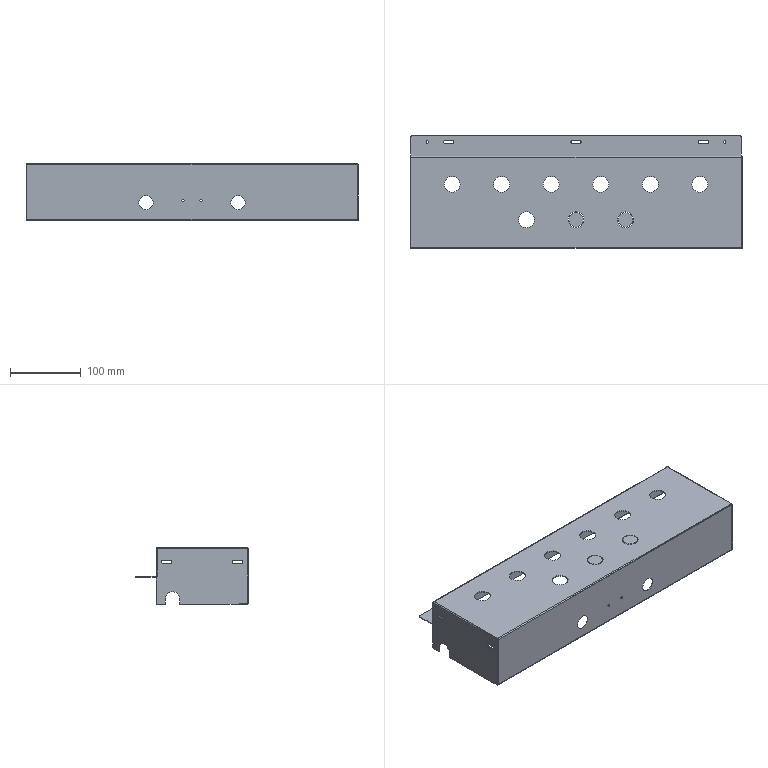Part | STEP file | 1 solid | 163 faces | box 469 x 158.8 x 80 mm | volume 180608 mm3 | cylinder 85 | plane 78 | commonest cylinder face diameters 22.5 x22 4.5 x17 3.3 x14 20.5 x8 0.4 x6 2.8 x6